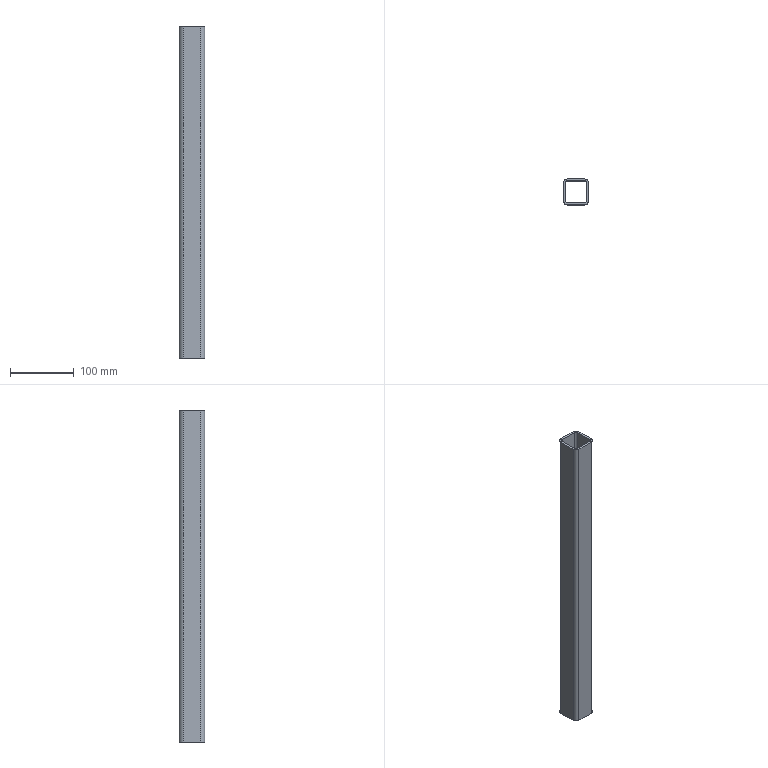Part | STEP file | 3 | 1 solid | 18 faces | box 40 x 40 x 520 mm | volume 217221 mm3 | plane 10 | cylinder 8 | commonest cylinder face diameters 7.2 x4 13.2 x4
STEP:
#1=CARTESIAN_POINT('',(0.,0.,0.));
#2=DIRECTION('',(0.,0.,1.));
#3=DIRECTION('',(1.,0.,0.));
#4=AXIS2_PLACEMENT_3D('',#1,#2,#3);
#5=CARTESIAN_POINT('',(-13.4,-17.,520.));
#6=VERTEX_POINT('',#5);
#7=CARTESIAN_POINT('',(13.4,-17.,520.));
#8=VERTEX_POINT('',#7);
#9=CARTESIAN_POINT('',(6.7,-17.,520.));
#10=DIRECTION('',(1.,0.,0.));
#11=VECTOR('',#10,1.);
#12=LINE('',#9,#11);
#13=CARTESIAN_POINT('',(13.4,-17.,0.));
#14=DIRECTION('',(0.,-1.,0.));
#15=DIRECTION('',(0.,0.,-1.));
#16=AXIS2_PLACEMENT_3D('',#13,#14,#15);
#17=PLANE('',#16);
#18=CARTESIAN_POINT('',(-520.,-6.7));
#19=DIRECTION('',(0.,1.));
#20=VECTOR('',#19,1.);
#21=LINE('',#18,#20);
#22=(GEOMETRIC_REPRESENTATION_CONTEXT(2)PARAMETRIC_REPRESENTATION_CONTEXT()REPRESENTATION_CONTEXT('',''));
#23=DEFINITIONAL_REPRESENTATION('',(#21),#22);
#24=PCURVE('',#17,#23);
#25=CARTESIAN_POINT('',(0.,0.,520.));
#26=DIRECTION('',(0.,0.,1.));
#27=DIRECTION('',(1.,0.,0.));
#28=AXIS2_PLACEMENT_3D('',#25,#26,#27);
#29=PLANE('',#28);
#30=CARTESIAN_POINT('',(6.7,-17.));
#31=DIRECTION('',(1.,0.));
#32=VECTOR('',#31,1.);
#33=LINE('',#30,#32);
#34=(GEOMETRIC_REPRESENTATION_CONTEXT(2)PARAMETRIC_REPRESENTATION_CONTEXT()REPRESENTATION_CONTEXT('',''));
#35=DEFINITIONAL_REPRESENTATION('',(#33),#34);
#36=PCURVE('',#29,#35);
#37=SURFACE_CURVE('',#12,(#24,#36),.PCURVE_S1.);
#38=EDGE_CURVE('',#6,#8,#37,.T.);
#39=ORIENTED_EDGE('',*,*,#38,.T.);
#40=CARTESIAN_POINT('',(13.4,-17.,0.));
#41=VERTEX_POINT('',#40);
#42=CARTESIAN_POINT('',(13.4,-17.,0.));
#43=DIRECTION('',(0.,0.,1.));
#44=VECTOR('',#43,1.);
#45=LINE('',#42,#44);
#46=CARTESIAN_POINT('',(0.,0.));
#47=DIRECTION('',(-1.,0.));
#48=VECTOR('',#47,1.);
#49=LINE('',#46,#48);
#50=(GEOMETRIC_REPRESENTATION_CONTEXT(2)PARAMETRIC_REPRESENTATION_CONTEXT()REPRESENTATION_CONTEXT('',''));
#51=DEFINITIONAL_REPRESENTATION('',(#49),#50);
#52=PCURVE('',#17,#51);
#53=CARTESIAN_POINT('',(13.4,-13.4,0.));
#54=DIRECTION('',(0.,0.,1.));
#55=DIRECTION('',(0.,1.,0.));
#56=AXIS2_PLACEMENT_3D('',#53,#54,#55);
#57=CYLINDRICAL_SURFACE('',#56,3.6);
#58=CARTESIAN_POINT('',(3.142,0.));
#59=DIRECTION('',(0.,1.));
#60=VECTOR('',#59,1.);
#61=LINE('',#58,#60);
#62=(GEOMETRIC_REPRESENTATION_CONTEXT(2)PARAMETRIC_REPRESENTATION_CONTEXT()REPRESENTATION_CONTEXT('',''));
#63=DEFINITIONAL_REPRESENTATION('',(#61),#62);
#64=PCURVE('',#57,#63);
#65=SURFACE_CURVE('',#45,(#52,#64),.PCURVE_S1.);
#66=EDGE_CURVE('',#41,#8,#65,.T.);
#67=ORIENTED_EDGE('',*,*,#66,.F.);
#68=CARTESIAN_POINT('',(-13.4,-17.,0.));
#69=VERTEX_POINT('',#68);
#70=CARTESIAN_POINT('',(6.7,-17.,0.));
#71=DIRECTION('',(1.,0.,0.));
#72=VECTOR('',#71,1.);
#73=LINE('',#70,#72);
#74=CARTESIAN_POINT('',(0.,-6.7));
#75=DIRECTION('',(0.,1.));
#76=VECTOR('',#75,1.);
#77=LINE('',#74,#76);
#78=(GEOMETRIC_REPRESENTATION_CONTEXT(2)PARAMETRIC_REPRESENTATION_CONTEXT()REPRESENTATION_CONTEXT('',''));
#79=DEFINITIONAL_REPRESENTATION('',(#77),#78);
#80=PCURVE('',#17,#79);
#81=CARTESIAN_POINT('',(0.,0.,0.));
#82=DIRECTION('',(0.,0.,1.));
#83=DIRECTION('',(1.,0.,0.));
#84=AXIS2_PLACEMENT_3D('',#81,#82,#83);
#85=PLANE('',#84);
#86=CARTESIAN_POINT('',(6.7,-17.));
#87=DIRECTION('',(1.,0.));
#88=VECTOR('',#87,1.);
#89=LINE('',#86,#88);
#90=(GEOMETRIC_REPRESENTATION_CONTEXT(2)PARAMETRIC_REPRESENTATION_CONTEXT()REPRESENTATION_CONTEXT('',''));
#91=DEFINITIONAL_REPRESENTATION('',(#89),#90);
#92=PCURVE('',#85,#91);
#93=SURFACE_CURVE('',#73,(#80,#92),.PCURVE_S1.);
#94=EDGE_CURVE('',#69,#41,#93,.T.);
#95=ORIENTED_EDGE('',*,*,#94,.F.);
#96=CARTESIAN_POINT('',(-13.4,-17.,0.));
#97=DIRECTION('',(0.,0.,1.));
#98=VECTOR('',#97,1.);
#99=LINE('',#96,#98);
#100=CARTESIAN_POINT('',(0.,-26.8));
#101=DIRECTION('',(-1.,0.));
#102=VECTOR('',#101,1.);
#103=LINE('',#100,#102);
#104=(GEOMETRIC_REPRESENTATION_CONTEXT(2)PARAMETRIC_REPRESENTATION_CONTEXT()REPRESENTATION_CONTEXT('',''));
#105=DEFINITIONAL_REPRESENTATION('',(#103),#104);
#106=PCURVE('',#17,#105);
#107=CARTESIAN_POINT('',(-13.4,-13.4,0.));
#108=DIRECTION('',(0.,0.,1.));
#109=DIRECTION('',(1.,0.,0.));
#110=AXIS2_PLACEMENT_3D('',#107,#108,#109);
#111=CYLINDRICAL_SURFACE('',#110,3.6);
#112=CARTESIAN_POINT('',(4.712,0.));
#113=DIRECTION('',(0.,1.));
#114=VECTOR('',#113,1.);
#115=LINE('',#112,#114);
#116=(GEOMETRIC_REPRESENTATION_CONTEXT(2)PARAMETRIC_REPRESENTATION_CONTEXT()REPRESENTATION_CONTEXT('',''));
#117=DEFINITIONAL_REPRESENTATION('',(#115),#116);
#118=PCURVE('',#111,#117);
#119=SURFACE_CURVE('',#99,(#106,#118),.PCURVE_S1.);
#120=EDGE_CURVE('',#69,#6,#119,.T.);
#121=ORIENTED_EDGE('',*,*,#120,.T.);
#122=EDGE_LOOP('',(#39,#67,#95,#121));
#123=FACE_BOUND('',#122,.T.);
#124=ADVANCED_FACE('',(#123),#17,.F.);
#125=ORIENTED_EDGE('',*,*,#66,.F.);
#126=CARTESIAN_POINT('',(17.,-13.4,0.));
#127=VERTEX_POINT('',#126);
#128=CARTESIAN_POINT('',(13.4,-13.4,0.));
#129=DIRECTION('',(0.,0.,1.));
#130=DIRECTION('',(0.,1.,0.));
#131=AXIS2_PLACEMENT_3D('',#128,#129,#130);
#132=CIRCLE('',#131,3.6);
#133=CARTESIAN_POINT('',(0.,0.));
#134=DIRECTION('',(1.,0.));
#135=VECTOR('',#134,1.);
#136=LINE('',#133,#135);
#137=(GEOMETRIC_REPRESENTATION_CONTEXT(2)PARAMETRIC_REPRESENTATION_CONTEXT()REPRESENTATION_CONTEXT('',''));
#138=DEFINITIONAL_REPRESENTATION('',(#136),#137);
#139=PCURVE('',#57,#138);
#140=CARTESIAN_POINT('',(13.4,-13.4));
#141=DIRECTION('',(0.,1.));
#142=AXIS2_PLACEMENT_2D('',#140,#141);
#143=CIRCLE('',#142,3.6);
#144=(GEOMETRIC_REPRESENTATION_CONTEXT(2)PARAMETRIC_REPRESENTATION_CONTEXT()REPRESENTATION_CONTEXT('',''));
#145=DEFINITIONAL_REPRESENTATION('',(#143),#144);
#146=PCURVE('',#85,#145);
#147=SURFACE_CURVE('',#132,(#139,#146),.PCURVE_S1.);
#148=EDGE_CURVE('',#41,#127,#147,.T.);
#149=ORIENTED_EDGE('',*,*,#148,.T.);
#150=CARTESIAN_POINT('',(17.,-13.4,520.));
#151=VERTEX_POINT('',#150);
#152=CARTESIAN_POINT('',(17.,-13.4,0.));
#153=DIRECTION('',(0.,0.,1.));
#154=VECTOR('',#153,1.);
#155=LINE('',#152,#154);
#156=CARTESIAN_POINT('',(4.712,0.));
#157=DIRECTION('',(0.,1.));
#158=VECTOR('',#157,1.);
#159=LINE('',#156,#158);
#160=(GEOMETRIC_REPRESENTATION_CONTEXT(2)PARAMETRIC_REPRESENTATION_CONTEXT()REPRESENTATION_CONTEXT('',''));
#161=DEFINITIONAL_REPRESENTATION('',(#159),#160);
#162=PCURVE('',#57,#161);
#163=CARTESIAN_POINT('',(17.,13.4,0.));
#164=DIRECTION('',(1.,0.,0.));
#165=DIRECTION('',(0.,0.,-1.));
#166=AXIS2_PLACEMENT_3D('',#163,#164,#165);
#167=PLANE('',#166);
#168=CARTESIAN_POINT('',(0.,-26.8));
#169=DIRECTION('',(-1.,0.));
#170=VECTOR('',#169,1.);
#171=LINE('',#168,#170);
#172=(GEOMETRIC_REPRESENTATION_CONTEXT(2)PARAMETRIC_REPRESENTATION_CONTEXT()REPRESENTATION_CONTEXT('',''));
#173=DEFINITIONAL_REPRESENTATION('',(#171),#172);
#174=PCURVE('',#167,#173);
#175=SURFACE_CURVE('',#155,(#162,#174),.PCURVE_S1.);
#176=EDGE_CURVE('',#127,#151,#175,.T.);
#177=ORIENTED_EDGE('',*,*,#176,.T.);
#178=CARTESIAN_POINT('',(13.4,-13.4,520.));
#179=DIRECTION('',(0.,0.,1.));
#180=DIRECTION('',(0.,1.,0.));
#181=AXIS2_PLACEMENT_3D('',#178,#179,#180);
#182=CIRCLE('',#181,3.6);
#183=CARTESIAN_POINT('',(0.,520.));
#184=DIRECTION('',(1.,0.));
#185=VECTOR('',#184,1.);
#186=LINE('',#183,#185);
#187=(GEOMETRIC_REPRESENTATION_CONTEXT(2)PARAMETRIC_REPRESENTATION_CONTEXT()REPRESENTATION_CONTEXT('',''));
#188=DEFINITIONAL_REPRESENTATION('',(#186),#187);
#189=PCURVE('',#57,#188);
#190=CARTESIAN_POINT('',(13.4,-13.4));
#191=DIRECTION('',(0.,1.));
#192=AXIS2_PLACEMENT_2D('',#190,#191);
#193=CIRCLE('',#192,3.6);
#194=(GEOMETRIC_REPRESENTATION_CONTEXT(2)PARAMETRIC_REPRESENTATION_CONTEXT()REPRESENTATION_CONTEXT('',''));
#195=DEFINITIONAL_REPRESENTATION('',(#193),#194);
#196=PCURVE('',#29,#195);
#197=SURFACE_CURVE('',#182,(#189,#196),.PCURVE_S1.);
#198=EDGE_CURVE('',#8,#151,#197,.T.);
#199=ORIENTED_EDGE('',*,*,#198,.F.);
#200=EDGE_LOOP('',(#125,#149,#177,#199));
#201=FACE_BOUND('',#200,.F.);
#202=ADVANCED_FACE('',(#201),#57,.F.);
#203=CARTESIAN_POINT('',(17.,13.4,520.));
#204=VERTEX_POINT('',#203);
#205=CARTESIAN_POINT('',(17.,6.7,520.));
#206=DIRECTION('',(0.,1.,0.));
#207=VECTOR('',#206,1.);
#208=LINE('',#205,#207);
#209=CARTESIAN_POINT('',(-520.,-6.7));
#210=DIRECTION('',(0.,1.));
#211=VECTOR('',#210,1.);
#212=LINE('',#209,#211);
#213=(GEOMETRIC_REPRESENTATION_CONTEXT(2)PARAMETRIC_REPRESENTATION_CONTEXT()REPRESENTATION_CONTEXT('',''));
#214=DEFINITIONAL_REPRESENTATION('',(#212),#213);
#215=PCURVE('',#167,#214);
#216=CARTESIAN_POINT('',(17.,6.7));
#217=DIRECTION('',(0.,1.));
#218=VECTOR('',#217,1.);
#219=LINE('',#216,#218);
#220=(GEOMETRIC_REPRESENTATION_CONTEXT(2)PARAMETRIC_REPRESENTATION_CONTEXT()REPRESENTATION_CONTEXT('',''));
#221=DEFINITIONAL_REPRESENTATION('',(#219),#220);
#222=PCURVE('',#29,#221);
#223=SURFACE_CURVE('',#208,(#215,#222),.PCURVE_S1.);
#224=EDGE_CURVE('',#151,#204,#223,.T.);
#225=ORIENTED_EDGE('',*,*,#224,.T.);
#226=CARTESIAN_POINT('',(17.,13.4,0.));
#227=VERTEX_POINT('',#226);
#228=CARTESIAN_POINT('',(17.,13.4,0.));
#229=DIRECTION('',(0.,0.,1.));
#230=VECTOR('',#229,1.);
#231=LINE('',#228,#230);
#232=CARTESIAN_POINT('',(0.,0.));
#233=DIRECTION('',(-1.,0.));
#234=VECTOR('',#233,1.);
#235=LINE('',#232,#234);
#236=(GEOMETRIC_REPRESENTATION_CONTEXT(2)PARAMETRIC_REPRESENTATION_CONTEXT()REPRESENTATION_CONTEXT('',''));
#237=DEFINITIONAL_REPRESENTATION('',(#235),#236);
#238=PCURVE('',#167,#237);
#239=CARTESIAN_POINT('',(13.4,13.4,0.));
#240=DIRECTION('',(0.,0.,1.));
#241=DIRECTION('',(-1.,0.,0.));
#242=AXIS2_PLACEMENT_3D('',#239,#240,#241);
#243=CYLINDRICAL_SURFACE('',#242,3.6);
#244=CARTESIAN_POINT('',(3.142,0.));
#245=DIRECTION('',(0.,1.));
#246=VECTOR('',#245,1.);
#247=LINE('',#244,#246);
#248=(GEOMETRIC_REPRESENTATION_CONTEXT(2)PARAMETRIC_REPRESENTATION_CONTEXT()REPRESENTATION_CONTEXT('',''));
#249=DEFINITIONAL_REPRESENTATION('',(#247),#248);
#250=PCURVE('',#243,#249);
#251=SURFACE_CURVE('',#231,(#238,#250),.PCURVE_S1.);
#252=EDGE_CURVE('',#227,#204,#251,.T.);
#253=ORIENTED_EDGE('',*,*,#252,.F.);
#254=CARTESIAN_POINT('',(17.,6.7,0.));
#255=DIRECTION('',(0.,1.,0.));
#256=VECTOR('',#255,1.);
#257=LINE('',#254,#256);
#258=CARTESIAN_POINT('',(0.,-6.7));
#259=DIRECTION('',(0.,1.));
#260=VECTOR('',#259,1.);
#261=LINE('',#258,#260);
#262=(GEOMETRIC_REPRESENTATION_CONTEXT(2)PARAMETRIC_REPRESENTATION_CONTEXT()REPRESENTATION_CONTEXT('',''));
#263=DEFINITIONAL_REPRESENTATION('',(#261),#262);
#264=PCURVE('',#167,#263);
#265=CARTESIAN_POINT('',(17.,6.7));
#266=DIRECTION('',(0.,1.));
#267=VECTOR('',#266,1.);
#268=LINE('',#265,#267);
#269=(GEOMETRIC_REPRESENTATION_CONTEXT(2)PARAMETRIC_REPRESENTATION_CONTEXT()REPRESENTATION_CONTEXT('',''));
#270=DEFINITIONAL_REPRESENTATION('',(#268),#269);
#271=PCURVE('',#85,#270);
#272=SURFACE_CURVE('',#257,(#264,#271),.PCURVE_S1.);
#273=EDGE_CURVE('',#127,#227,#272,.T.);
#274=ORIENTED_EDGE('',*,*,#273,.F.);
#275=ORIENTED_EDGE('',*,*,#176,.T.);
#276=EDGE_LOOP('',(#225,#253,#274,#275));
#277=FACE_BOUND('',#276,.T.);
#278=ADVANCED_FACE('',(#277),#167,.F.);
#279=ORIENTED_EDGE('',*,*,#252,.F.);
#280=CARTESIAN_POINT('',(13.4,17.,0.));
#281=VERTEX_POINT('',#280);
#282=CARTESIAN_POINT('',(13.4,13.4,0.));
#283=DIRECTION('',(0.,0.,1.));
#284=DIRECTION('',(-1.,0.,0.));
#285=AXIS2_PLACEMENT_3D('',#282,#283,#284);
#286=CIRCLE('',#285,3.6);
#287=CARTESIAN_POINT('',(0.,0.));
#288=DIRECTION('',(1.,0.));
#289=VECTOR('',#288,1.);
#290=LINE('',#287,#289);
#291=(GEOMETRIC_REPRESENTATION_CONTEXT(2)PARAMETRIC_REPRESENTATION_CONTEXT()REPRESENTATION_CONTEXT('',''));
#292=DEFINITIONAL_REPRESENTATION('',(#290),#291);
#293=PCURVE('',#243,#292);
#294=CARTESIAN_POINT('',(13.4,13.4));
#295=DIRECTION('',(-1.,0.));
#296=AXIS2_PLACEMENT_2D('',#294,#295);
#297=CIRCLE('',#296,3.6);
#298=(GEOMETRIC_REPRESENTATION_CONTEXT(2)PARAMETRIC_REPRESENTATION_CONTEXT()REPRESENTATION_CONTEXT('',''));
#299=DEFINITIONAL_REPRESENTATION('',(#297),#298);
#300=PCURVE('',#85,#299);
#301=SURFACE_CURVE('',#286,(#293,#300),.PCURVE_S1.);
#302=EDGE_CURVE('',#227,#281,#301,.T.);
#303=ORIENTED_EDGE('',*,*,#302,.T.);
#304=CARTESIAN_POINT('',(13.4,17.,520.));
#305=VERTEX_POINT('',#304);
#306=CARTESIAN_POINT('',(13.4,17.,0.));
#307=DIRECTION('',(0.,0.,1.));
#308=VECTOR('',#307,1.);
#309=LINE('',#306,#308);
#310=CARTESIAN_POINT('',(4.712,0.));
#311=DIRECTION('',(0.,1.));
#312=VECTOR('',#311,1.);
#313=LINE('',#310,#312);
#314=(GEOMETRIC_REPRESENTATION_CONTEXT(2)PARAMETRIC_REPRESENTATION_CONTEXT()REPRESENTATION_CONTEXT('',''));
#315=DEFINITIONAL_REPRESENTATION('',(#313),#314);
#316=PCURVE('',#243,#315);
#317=CARTESIAN_POINT('',(-13.4,17.,0.));
#318=DIRECTION('',(0.,1.,0.));
#319=DIRECTION('',(0.,0.,1.));
#320=AXIS2_PLACEMENT_3D('',#317,#318,#319);
#321=PLANE('',#320);
#322=CARTESIAN_POINT('',(0.,26.8));
#323=DIRECTION('',(1.,0.));
#324=VECTOR('',#323,1.);
#325=LINE('',#322,#324);
#326=(GEOMETRIC_REPRESENTATION_CONTEXT(2)PARAMETRIC_REPRESENTATION_CONTEXT()REPRESENTATION_CONTEXT('',''));
#327=DEFINITIONAL_REPRESENTATION('',(#325),#326);
#328=PCURVE('',#321,#327);
#329=SURFACE_CURVE('',#309,(#316,#328),.PCURVE_S1.);
#330=EDGE_CURVE('',#281,#305,#329,.T.);
#331=ORIENTED_EDGE('',*,*,#330,.T.);
#332=CARTESIAN_POINT('',(13.4,13.4,520.));
#333=DIRECTION('',(0.,0.,1.));
#334=DIRECTION('',(-1.,0.,0.));
#335=AXIS2_PLACEMENT_3D('',#332,#333,#334);
#336=CIRCLE('',#335,3.6);
#337=CARTESIAN_POINT('',(0.,520.));
#338=DIRECTION('',(1.,0.));
#339=VECTOR('',#338,1.);
#340=LINE('',#337,#339);
#341=(GEOMETRIC_REPRESENTATION_CONTEXT(2)PARAMETRIC_REPRESENTATION_CONTEXT()REPRESENTATION_CONTEXT('',''));
#342=DEFINITIONAL_REPRESENTATION('',(#340),#341);
#343=PCURVE('',#243,#342);
#344=CARTESIAN_POINT('',(13.4,13.4));
#345=DIRECTION('',(-1.,0.));
#346=AXIS2_PLACEMENT_2D('',#344,#345);
#347=CIRCLE('',#346,3.6);
#348=(GEOMETRIC_REPRESENTATION_CONTEXT(2)PARAMETRIC_REPRESENTATION_CONTEXT()REPRESENTATION_CONTEXT('',''));
#349=DEFINITIONAL_REPRESENTATION('',(#347),#348);
#350=PCURVE('',#29,#349);
#351=SURFACE_CURVE('',#336,(#343,#350),.PCURVE_S1.);
#352=EDGE_CURVE('',#204,#305,#351,.T.);
#353=ORIENTED_EDGE('',*,*,#352,.F.);
#354=EDGE_LOOP('',(#279,#303,#331,#353));
#355=FACE_BOUND('',#354,.F.);
#356=ADVANCED_FACE('',(#355),#243,.F.);
#357=CARTESIAN_POINT('',(20.,13.4,520.));
#358=VERTEX_POINT('',#357);
#359=CARTESIAN_POINT('',(20.,-13.4,520.));
#360=VERTEX_POINT('',#359);
#361=CARTESIAN_POINT('',(20.,6.7,520.));
#362=DIRECTION('',(0.,-1.,0.));
#363=VECTOR('',#362,1.);
#364=LINE('',#361,#363);
#365=CARTESIAN_POINT('',(20.,13.4,0.));
#366=DIRECTION('',(1.,0.,0.));
#367=DIRECTION('',(0.,0.,-1.));
#368=AXIS2_PLACEMENT_3D('',#365,#366,#367);
#369=PLANE('',#368);
#370=CARTESIAN_POINT('',(-520.,-6.7));
#371=DIRECTION('',(0.,-1.));
#372=VECTOR('',#371,1.);
#373=LINE('',#370,#372);
#374=(GEOMETRIC_REPRESENTATION_CONTEXT(2)PARAMETRIC_REPRESENTATION_CONTEXT()REPRESENTATION_CONTEXT('',''));
#375=DEFINITIONAL_REPRESENTATION('',(#373),#374);
#376=PCURVE('',#369,#375);
#377=CARTESIAN_POINT('',(20.,6.7));
#378=DIRECTION('',(0.,-1.));
#379=VECTOR('',#378,1.);
#380=LINE('',#377,#379);
#381=(GEOMETRIC_REPRESENTATION_CONTEXT(2)PARAMETRIC_REPRESENTATION_CONTEXT()REPRESENTATION_CONTEXT('',''));
#382=DEFINITIONAL_REPRESENTATION('',(#380),#381);
#383=PCURVE('',#29,#382);
#384=SURFACE_CURVE('',#364,(#376,#383),.PCURVE_S1.);
#385=EDGE_CURVE('',#358,#360,#384,.T.);
#386=ORIENTED_EDGE('',*,*,#385,.T.);
#387=CARTESIAN_POINT('',(20.,-13.4,0.));
#388=VERTEX_POINT('',#387);
#389=CARTESIAN_POINT('',(20.,-13.4,0.));
#390=DIRECTION('',(0.,0.,1.));
#391=VECTOR('',#390,1.);
#392=LINE('',#389,#391);
#393=CARTESIAN_POINT('',(0.,-26.8));
#394=DIRECTION('',(-1.,0.));
#395=VECTOR('',#394,1.);
#396=LINE('',#393,#395);
#397=(GEOMETRIC_REPRESENTATION_CONTEXT(2)PARAMETRIC_REPRESENTATION_CONTEXT()REPRESENTATION_CONTEXT('',''));
#398=DEFINITIONAL_REPRESENTATION('',(#396),#397);
#399=PCURVE('',#369,#398);
#400=CARTESIAN_POINT('',(13.4,-13.4,0.));
#401=DIRECTION('',(0.,0.,1.));
#402=DIRECTION('',(0.,1.,0.));
#403=AXIS2_PLACEMENT_3D('',#400,#401,#402);
#404=CYLINDRICAL_SURFACE('',#403,6.6);
#405=CARTESIAN_POINT('',(4.712,0.));
#406=DIRECTION('',(0.,1.));
#407=VECTOR('',#406,1.);
#408=LINE('',#405,#407);
#409=(GEOMETRIC_REPRESENTATION_CONTEXT(2)PARAMETRIC_REPRESENTATION_CONTEXT()REPRESENTATION_CONTEXT('',''));
#410=DEFINITIONAL_REPRESENTATION('',(#408),#409);
#411=PCURVE('',#404,#410);
#412=SURFACE_CURVE('',#392,(#399,#411),.PCURVE_S1.);
#413=EDGE_CURVE('',#388,#360,#412,.T.);
#414=ORIENTED_EDGE('',*,*,#413,.F.);
#415=CARTESIAN_POINT('',(20.,13.4,0.));
#416=VERTEX_POINT('',#415);
#417=CARTESIAN_POINT('',(20.,6.7,0.));
#418=DIRECTION('',(0.,-1.,0.));
#419=VECTOR('',#418,1.);
#420=LINE('',#417,#419);
#421=CARTESIAN_POINT('',(0.,-6.7));
#422=DIRECTION('',(0.,-1.));
#423=VECTOR('',#422,1.);
#424=LINE('',#421,#423);
#425=(GEOMETRIC_REPRESENTATION_CONTEXT(2)PARAMETRIC_REPRESENTATION_CONTEXT()REPRESENTATION_CONTEXT('',''));
#426=DEFINITIONAL_REPRESENTATION('',(#424),#425);
#427=PCURVE('',#369,#426);
#428=CARTESIAN_POINT('',(20.,6.7));
#429=DIRECTION('',(0.,-1.));
#430=VECTOR('',#429,1.);
#431=LINE('',#428,#430);
#432=(GEOMETRIC_REPRESENTATION_CONTEXT(2)PARAMETRIC_REPRESENTATION_CONTEXT()REPRESENTATION_CONTEXT('',''));
#433=DEFINITIONAL_REPRESENTATION('',(#431),#432);
#434=PCURVE('',#85,#433);
#435=SURFACE_CURVE('',#420,(#427,#434),.PCURVE_S1.);
#436=EDGE_CURVE('',#416,#388,#435,.T.);
#437=ORIENTED_EDGE('',*,*,#436,.F.);
#438=CARTESIAN_POINT('',(20.,13.4,0.));
#439=DIRECTION('',(0.,0.,1.));
#440=VECTOR('',#439,1.);
#441=LINE('',#438,#440);
#442=CARTESIAN_POINT('',(0.,0.));
#443=DIRECTION('',(-1.,0.));
#444=VECTOR('',#443,1.);
#445=LINE('',#442,#444);
#446=(GEOMETRIC_REPRESENTATION_CONTEXT(2)PARAMETRIC_REPRESENTATION_CONTEXT()REPRESENTATION_CONTEXT('',''));
#447=DEFINITIONAL_REPRESENTATION('',(#445),#446);
#448=PCURVE('',#369,#447);
#449=CARTESIAN_POINT('',(13.4,13.4,0.));
#450=DIRECTION('',(0.,0.,1.));
#451=DIRECTION('',(-1.,0.,0.));
#452=AXIS2_PLACEMENT_3D('',#449,#450,#451);
#453=CYLINDRICAL_SURFACE('',#452,6.6);
#454=CARTESIAN_POINT('',(3.142,0.));
#455=DIRECTION('',(0.,1.));
#456=VECTOR('',#455,1.);
#457=LINE('',#454,#456);
#458=(GEOMETRIC_REPRESENTATION_CONTEXT(2)PARAMETRIC_REPRESENTATION_CONTEXT()REPRESENTATION_CONTEXT('',''));
#459=DEFINITIONAL_REPRESENTATION('',(#457),#458);
#460=PCURVE('',#453,#459);
#461=SURFACE_CURVE('',#441,(#448,#460),.PCURVE_S1.);
#462=EDGE_CURVE('',#416,#358,#461,.T.);
#463=ORIENTED_EDGE('',*,*,#462,.T.);
#464=EDGE_LOOP('',(#386,#414,#437,#463));
#465=FACE_BOUND('',#464,.T.);
#466=ADVANCED_FACE('',(#465),#369,.T.);
#467=CARTESIAN_POINT('',(13.4,-20.,520.));
#468=VERTEX_POINT('',#467);
#469=CARTESIAN_POINT('',(13.4,-13.4,520.));
#470=DIRECTION('',(0.,0.,-1.));
#471=DIRECTION('',(0.,1.,0.));
#472=AXIS2_PLACEMENT_3D('',#469,#470,#471);
#473=CIRCLE('',#472,6.6);
#474=CARTESIAN_POINT('',(6.283,520.));
#475=DIRECTION('',(-1.,0.));
#476=VECTOR('',#475,1.);
#477=LINE('',#474,#476);
#478=(GEOMETRIC_REPRESENTATION_CONTEXT(2)PARAMETRIC_REPRESENTATION_CONTEXT()REPRESENTATION_CONTEXT('',''));
#479=DEFINITIONAL_REPRESENTATION('',(#477),#478);
#480=PCURVE('',#404,#479);
#481=CARTESIAN_POINT('',(13.4,-6.8));
#482=CARTESIAN_POINT('',(24.832,-6.8));
#483=CARTESIAN_POINT('',(19.116,-16.7));
#484=CARTESIAN_POINT('',(13.4,-26.6));
#485=CARTESIAN_POINT('',(7.684,-16.7));
#486=CARTESIAN_POINT('',(1.968,-6.8));
#487=CARTESIAN_POINT('',(13.4,-6.8));
#488=(BOUNDED_CURVE()B_SPLINE_CURVE(2,(#481,#482,#483,#484,#485,#486,#487),.UNSPECIFIED.,.T.,.F.)B_SPLINE_CURVE_WITH_KNOTS((1,2,2,2,2,1),(-2.094,0.,2.094,4.189,6.283,8.378),.UNSPECIFIED.)CURVE()GEOMETRIC_REPRESENTATION_ITEM()RATIONAL_B_SPLINE_CURVE((1.,0.5,1.,0.5,1.,0.5,1.))REPRESENTATION_ITEM(''));
#489=(GEOMETRIC_REPRESENTATION_CONTEXT(2)PARAMETRIC_REPRESENTATION_CONTEXT()REPRESENTATION_CONTEXT('',''));
#490=DEFINITIONAL_REPRESENTATION('',(#488),#489);
#491=PCURVE('',#29,#490);
#492=SURFACE_CURVE('',#473,(#480,#491),.PCURVE_S1.);
#493=EDGE_CURVE('',#360,#468,#492,.T.);
#494=ORIENTED_EDGE('',*,*,#493,.T.);
#495=CARTESIAN_POINT('',(13.4,-20.,0.));
#496=VERTEX_POINT('',#495);
#497=CARTESIAN_POINT('',(13.4,-20.,0.));
#498=DIRECTION('',(0.,0.,1.));
#499=VECTOR('',#498,1.);
#500=LINE('',#497,#499);
#501=CARTESIAN_POINT('',(3.142,0.));
#502=DIRECTION('',(0.,1.));
#503=VECTOR('',#502,1.);
#504=LINE('',#501,#503);
#505=(GEOMETRIC_REPRESENTATION_CONTEXT(2)PARAMETRIC_REPRESENTATION_CONTEXT()REPRESENTATION_CONTEXT('',''));
#506=DEFINITIONAL_REPRESENTATION('',(#504),#505);
#507=PCURVE('',#404,#506);
#508=CARTESIAN_POINT('',(13.4,-20.,0.));
#509=DIRECTION('',(0.,-1.,0.));
#510=DIRECTION('',(0.,0.,-1.));
#511=AXIS2_PLACEMENT_3D('',#508,#509,#510);
#512=PLANE('',#511);
#513=CARTESIAN_POINT('',(0.,0.));
#514=DIRECTION('',(-1.,0.));
#515=VECTOR('',#514,1.);
#516=LINE('',#513,#515);
#517=(GEOMETRIC_REPRESENTATION_CONTEXT(2)PARAMETRIC_REPRESENTATION_CONTEXT()REPRESENTATION_CONTEXT('',''));
#518=DEFINITIONAL_REPRESENTATION('',(#516),#517);
#519=PCURVE('',#512,#518);
#520=SURFACE_CURVE('',#500,(#507,#519),.PCURVE_S1.);
#521=EDGE_CURVE('',#496,#468,#520,.T.);
#522=ORIENTED_EDGE('',*,*,#521,.F.);
#523=CARTESIAN_POINT('',(13.4,-13.4,0.));
#524=DIRECTION('',(0.,0.,-1.));
#525=DIRECTION('',(0.,1.,0.));
#526=AXIS2_PLACEMENT_3D('',#523,#524,#525);
#527=CIRCLE('',#526,6.6);
#528=CARTESIAN_POINT('',(6.283,0.));
#529=DIRECTION('',(-1.,0.));
#530=VECTOR('',#529,1.);
#531=LINE('',#528,#530);
#532=(GEOMETRIC_REPRESENTATION_CONTEXT(2)PARAMETRIC_REPRESENTATION_CONTEXT()REPRESENTATION_CONTEXT('',''));
#533=DEFINITIONAL_REPRESENTATION('',(#531),#532);
#534=PCURVE('',#404,#533);
#535=CARTESIAN_POINT('',(13.4,-6.8));
#536=CARTESIAN_POINT('',(24.832,-6.8));
#537=CARTESIAN_POINT('',(19.116,-16.7));
#538=CARTESIAN_POINT('',(13.4,-26.6));
#539=CARTESIAN_POINT('',(7.684,-16.7));
#540=CARTESIAN_POINT('',(1.968,-6.8));
#541=CARTESIAN_POINT('',(13.4,-6.8));
#542=(BOUNDED_CURVE()B_SPLINE_CURVE(2,(#535,#536,#537,#538,#539,#540,#541),.UNSPECIFIED.,.T.,.F.)B_SPLINE_CURVE_WITH_KNOTS((1,2,2,2,2,1),(-2.094,0.,2.094,4.189,6.283,8.378),.UNSPECIFIED.)CURVE()GEOMETRIC_REPRESENTATION_ITEM()RATIONAL_B_SPLINE_CURVE((1.,0.5,1.,0.5,1.,0.5,1.))REPRESENTATION_ITEM(''));
#543=(GEOMETRIC_REPRESENTATION_CONTEXT(2)PARAMETRIC_REPRESENTATION_CONTEXT()REPRESENTATION_CONTEXT('',''));
#544=DEFINITIONAL_REPRESENTATION('',(#542),#543);
#545=PCURVE('',#85,#544);
#546=SURFACE_CURVE('',#527,(#534,#545),.PCURVE_S1.);
#547=EDGE_CURVE('',#388,#496,#546,.T.);
#548=ORIENTED_EDGE('',*,*,#547,.F.);
#549=ORIENTED_EDGE('',*,*,#413,.T.);
#550=EDGE_LOOP('',(#494,#522,#548,#549));
#551=FACE_BOUND('',#550,.T.);
#552=ADVANCED_FACE('',(#551),#404,.T.);
#553=CARTESIAN_POINT('',(-13.4,-20.,520.));
#554=VERTEX_POINT('',#553);
#555=CARTESIAN_POINT('',(6.7,-20.,520.));
#556=DIRECTION('',(-1.,0.,0.));
#557=VECTOR('',#556,1.);
#558=LINE('',#555,#557);
#559=CARTESIAN_POINT('',(-520.,-6.7));
#560=DIRECTION('',(0.,-1.));
#561=VECTOR('',#560,1.);
#562=LINE('',#559,#561);
#563=(GEOMETRIC_REPRESENTATION_CONTEXT(2)PARAMETRIC_REPRESENTATION_CONTEXT()REPRESENTATION_CONTEXT('',''));
#564=DEFINITIONAL_REPRESENTATION('',(#562),#563);
#565=PCURVE('',#512,#564);
#566=CARTESIAN_POINT('',(6.7,-20.));
#567=DIRECTION('',(-1.,0.));
#568=VECTOR('',#567,1.);
#569=LINE('',#566,#568);
#570=(GEOMETRIC_REPRESENTATION_CONTEXT(2)PARAMETRIC_REPRESENTATION_CONTEXT()REPRESENTATION_CONTEXT('',''));
#571=DEFINITIONAL_REPRESENTATION('',(#569),#570);
#572=PCURVE('',#29,#571);
#573=SURFACE_CURVE('',#558,(#565,#572),.PCURVE_S1.);
#574=EDGE_CURVE('',#468,#554,#573,.T.);
#575=ORIENTED_EDGE('',*,*,#574,.T.);
#576=CARTESIAN_POINT('',(-13.4,-20.,0.));
#577=VERTEX_POINT('',#576);
#578=CARTESIAN_POINT('',(-13.4,-20.,0.));
#579=DIRECTION('',(0.,0.,1.));
#580=VECTOR('',#579,1.);
#581=LINE('',#578,#580);
#582=CARTESIAN_POINT('',(0.,-26.8));
#583=DIRECTION('',(-1.,0.));
#584=VECTOR('',#583,1.);
#585=LINE('',#582,#584);
#586=(GEOMETRIC_REPRESENTATION_CONTEXT(2)PARAMETRIC_REPRESENTATION_CONTEXT()REPRESENTATION_CONTEXT('',''));
#587=DEFINITIONAL_REPRESENTATION('',(#585),#586);
#588=PCURVE('',#512,#587);
#589=CARTESIAN_POINT('',(-13.4,-13.4,0.));
#590=DIRECTION('',(0.,0.,1.));
#591=DIRECTION('',(1.,0.,0.));
#592=AXIS2_PLACEMENT_3D('',#589,#590,#591);
#593=CYLINDRICAL_SURFACE('',#592,6.6);
#594=CARTESIAN_POINT('',(4.712,0.));
#595=DIRECTION('',(0.,1.));
#596=VECTOR('',#595,1.);
#597=LINE('',#594,#596);
#598=(GEOMETRIC_REPRESENTATION_CONTEXT(2)PARAMETRIC_REPRESENTATION_CONTEXT()REPRESENTATION_CONTEXT('',''));
#599=DEFINITIONAL_REPRESENTATION('',(#597),#598);
#600=PCURVE('',#593,#599);
#601=SURFACE_CURVE('',#581,(#588,#600),.PCURVE_S1.);
#602=EDGE_CURVE('',#577,#554,#601,.T.);
#603=ORIENTED_EDGE('',*,*,#602,.F.);
#604=CARTESIAN_POINT('',(6.7,-20.,0.));
#605=DIRECTION('',(-1.,0.,0.));
#606=VECTOR('',#605,1.);
#607=LINE('',#604,#606);
#608=CARTESIAN_POINT('',(0.,-6.7));
#609=DIRECTION('',(0.,-1.));
#610=VECTOR('',#609,1.);
#611=LINE('',#608,#610);
#612=(GEOMETRIC_REPRESENTATION_CONTEXT(2)PARAMETRIC_REPRESENTATION_CONTEXT()REPRESENTATION_CONTEXT('',''));
#613=DEFINITIONAL_REPRESENTATION('',(#611),#612);
#614=PCURVE('',#512,#613);
#615=CARTESIAN_POINT('',(6.7,-20.));
#616=DIRECTION('',(-1.,0.));
#617=VECTOR('',#616,1.);
#618=LINE('',#615,#617);
#619=(GEOMETRIC_REPRESENTATION_CONTEXT(2)PARAMETRIC_REPRESENTATION_CONTEXT()REPRESENTATION_CONTEXT('',''));
#620=DEFINITIONAL_REPRESENTATION('',(#618),#619);
#621=PCURVE('',#85,#620);
#622=SURFACE_CURVE('',#607,(#614,#621),.PCURVE_S1.);
#623=EDGE_CURVE('',#496,#577,#622,.T.);
#624=ORIENTED_EDGE('',*,*,#623,.F.);
#625=ORIENTED_EDGE('',*,*,#521,.T.);
#626=EDGE_LOOP('',(#575,#603,#624,#625));
#627=FACE_BOUND('',#626,.T.);
#628=ADVANCED_FACE('',(#627),#512,.T.);
#629=CARTESIAN_POINT('',(-20.,-13.4,520.));
#630=VERTEX_POINT('',#629);
#631=CARTESIAN_POINT('',(-13.4,-13.4,520.));
#632=DIRECTION('',(0.,0.,-1.));
#633=DIRECTION('',(1.,0.,0.));
#634=AXIS2_PLACEMENT_3D('',#631,#632,#633);
#635=CIRCLE('',#634,6.6);
#636=CARTESIAN_POINT('',(6.283,520.));
#637=DIRECTION('',(-1.,0.));
#638=VECTOR('',#637,1.);
#639=LINE('',#636,#638);
#640=(GEOMETRIC_REPRESENTATION_CONTEXT(2)PARAMETRIC_REPRESENTATION_CONTEXT()REPRESENTATION_CONTEXT('',''));
#641=DEFINITIONAL_REPRESENTATION('',(#639),#640);
#642=PCURVE('',#593,#641);
#643=CARTESIAN_POINT('',(-6.8,-13.4));
#644=CARTESIAN_POINT('',(-6.8,-24.832));
#645=CARTESIAN_POINT('',(-16.7,-19.116));
#646=CARTESIAN_POINT('',(-26.6,-13.4));
#647=CARTESIAN_POINT('',(-16.7,-7.684));
#648=CARTESIAN_POINT('',(-6.8,-1.968));
#649=CARTESIAN_POINT('',(-6.8,-13.4));
#650=(BOUNDED_CURVE()B_SPLINE_CURVE(2,(#643,#644,#645,#646,#647,#648,#649),.UNSPECIFIED.,.T.,.F.)B_SPLINE_CURVE_WITH_KNOTS((1,2,2,2,2,1),(-2.094,0.,2.094,4.189,6.283,8.378),.UNSPECIFIED.)CURVE()GEOMETRIC_REPRESENTATION_ITEM()RATIONAL_B_SPLINE_CURVE((1.,0.5,1.,0.5,1.,0.5,1.))REPRESENTATION_ITEM(''));
#651=(GEOMETRIC_REPRESENTATION_CONTEXT(2)PARAMETRIC_REPRESENTATION_CONTEXT()REPRESENTATION_CONTEXT('',''));
#652=DEFINITIONAL_REPRESENTATION('',(#650),#651);
#653=PCURVE('',#29,#652);
#654=SURFACE_CURVE('',#635,(#642,#653),.PCURVE_S1.);
#655=EDGE_CURVE('',#554,#630,#654,.T.);
#656=ORIENTED_EDGE('',*,*,#655,.T.);
#657=CARTESIAN_POINT('',(-20.,-13.4,0.));
#658=VERTEX_POINT('',#657);
#659=CARTESIAN_POINT('',(-20.,-13.4,0.));
#660=DIRECTION('',(0.,0.,1.));
#661=VECTOR('',#660,1.);
#662=LINE('',#659,#661);
#663=CARTESIAN_POINT('',(3.142,0.));
#664=DIRECTION('',(0.,1.));
#665=VECTOR('',#664,1.);
#666=LINE('',#663,#665);
#667=(GEOMETRIC_REPRESENTATION_CONTEXT(2)PARAMETRIC_REPRESENTATION_CONTEXT()REPRESENTATION_CONTEXT('',''));
#668=DEFINITIONAL_REPRESENTATION('',(#666),#667);
#669=PCURVE('',#593,#668);
#670=CARTESIAN_POINT('',(-20.,-13.4,0.));
#671=DIRECTION('',(-1.,0.,0.));
#672=DIRECTION('',(0.,0.,1.));
#673=AXIS2_PLACEMENT_3D('',#670,#671,#672);
#674=PLANE('',#673);
#675=CARTESIAN_POINT('',(0.,0.));
#676=DIRECTION('',(1.,0.));
#677=VECTOR('',#676,1.);
#678=LINE('',#675,#677);
#679=(GEOMETRIC_REPRESENTATION_CONTEXT(2)PARAMETRIC_REPRESENTATION_CONTEXT()REPRESENTATION_CONTEXT('',''));
#680=DEFINITIONAL_REPRESENTATION('',(#678),#679);
#681=PCURVE('',#674,#680);
#682=SURFACE_CURVE('',#662,(#669,#681),.PCURVE_S1.);
#683=EDGE_CURVE('',#658,#630,#682,.T.);
#684=ORIENTED_EDGE('',*,*,#683,.F.);
#685=CARTESIAN_POINT('',(-13.4,-13.4,0.));
#686=DIRECTION('',(0.,0.,-1.));
#687=DIRECTION('',(1.,0.,0.));
#688=AXIS2_PLACEMENT_3D('',#685,#686,#687);
#689=CIRCLE('',#688,6.6);
#690=CARTESIAN_POINT('',(6.283,0.));
#691=DIRECTION('',(-1.,0.));
#692=VECTOR('',#691,1.);
#693=LINE('',#690,#692);
#694=(GEOMETRIC_REPRESENTATION_CONTEXT(2)PARAMETRIC_REPRESENTATION_CONTEXT()REPRESENTATION_CONTEXT('',''));
#695=DEFINITIONAL_REPRESENTATION('',(#693),#694);
#696=PCURVE('',#593,#695);
#697=CARTESIAN_POINT('',(-6.8,-13.4));
#698=CARTESIAN_POINT('',(-6.8,-24.832));
#699=CARTESIAN_POINT('',(-16.7,-19.116));
#700=CARTESIAN_POINT('',(-26.6,-13.4));
#701=CARTESIAN_POINT('',(-16.7,-7.684));
#702=CARTESIAN_POINT('',(-6.8,-1.968));
#703=CARTESIAN_POINT('',(-6.8,-13.4));
#704=(BOUNDED_CURVE()B_SPLINE_CURVE(2,(#697,#698,#699,#700,#701,#702,#703),.UNSPECIFIED.,.T.,.F.)B_SPLINE_CURVE_WITH_KNOTS((1,2,2,2,2,1),(-2.094,0.,2.094,4.189,6.283,8.378),.UNSPECIFIED.)CURVE()GEOMETRIC_REPRESENTATION_ITEM()RATIONAL_B_SPLINE_CURVE((1.,0.5,1.,0.5,1.,0.5,1.))REPRESENTATION_ITEM(''));
#705=(GEOMETRIC_REPRESENTATION_CONTEXT(2)PARAMETRIC_REPRESENTATION_CONTEXT()REPRESENTATION_CONTEXT('',''));
#706=DEFINITIONAL_REPRESENTATION('',(#704),#705);
#707=PCURVE('',#85,#706);
#708=SURFACE_CURVE('',#689,(#696,#707),.PCURVE_S1.);
#709=EDGE_CURVE('',#577,#658,#708,.T.);
#710=ORIENTED_EDGE('',*,*,#709,.F.);
#711=ORIENTED_EDGE('',*,*,#602,.T.);
#712=EDGE_LOOP('',(#656,#684,#710,#711));
#713=FACE_BOUND('',#712,.T.);
#714=ADVANCED_FACE('',(#713),#593,.T.);
#715=CARTESIAN_POINT('',(-13.4,17.,520.));
#716=VERTEX_POINT('',#715);
#717=CARTESIAN_POINT('',(-6.7,17.,520.));
#718=DIRECTION('',(-1.,0.,0.));
#719=VECTOR('',#718,1.);
#720=LINE('',#717,#719);
#721=CARTESIAN_POINT('',(520.,6.7));
#722=DIRECTION('',(0.,-1.));
#723=VECTOR('',#722,1.);
#724=LINE('',#721,#723);
#725=(GEOMETRIC_REPRESENTATION_CONTEXT(2)PARAMETRIC_REPRESENTATION_CONTEXT()REPRESENTATION_CONTEXT('',''));
#726=DEFINITIONAL_REPRESENTATION('',(#724),#725);
#727=PCURVE('',#321,#726);
#728=CARTESIAN_POINT('',(-6.7,17.));
#729=DIRECTION('',(-1.,0.));
#730=VECTOR('',#729,1.);
#731=LINE('',#728,#730);
#732=(GEOMETRIC_REPRESENTATION_CONTEXT(2)PARAMETRIC_REPRESENTATION_CONTEXT()REPRESENTATION_CONTEXT('',''));
#733=DEFINITIONAL_REPRESENTATION('',(#731),#732);
#734=PCURVE('',#29,#733);
#735=SURFACE_CURVE('',#720,(#727,#734),.PCURVE_S1.);
#736=EDGE_CURVE('',#305,#716,#735,.T.);
#737=ORIENTED_EDGE('',*,*,#736,.T.);
#738=CARTESIAN_POINT('',(-13.4,17.,0.));
#739=VERTEX_POINT('',#738);
#740=CARTESIAN_POINT('',(-13.4,17.,0.));
#741=DIRECTION('',(0.,0.,1.));
#742=VECTOR('',#741,1.);
#743=LINE('',#740,#742);
#744=CARTESIAN_POINT('',(0.,0.));
#745=DIRECTION('',(1.,0.));
#746=VECTOR('',#745,1.);
#747=LINE('',#744,#746);
#748=(GEOMETRIC_REPRESENTATION_CONTEXT(2)PARAMETRIC_REPRESENTATION_CONTEXT()REPRESENTATION_CONTEXT('',''));
#749=DEFINITIONAL_REPRESENTATION('',(#747),#748);
#750=PCURVE('',#321,#749);
#751=CARTESIAN_POINT('',(-13.4,13.4,0.));
#752=DIRECTION('',(0.,0.,1.));
#753=DIRECTION('',(0.,-1.,0.));
#754=AXIS2_PLACEMENT_3D('',#751,#752,#753);
#755=CYLINDRICAL_SURFACE('',#754,3.6);
#756=CARTESIAN_POINT('',(3.142,0.));
#757=DIRECTION('',(0.,1.));
#758=VECTOR('',#757,1.);
#759=LINE('',#756,#758);
#760=(GEOMETRIC_REPRESENTATION_CONTEXT(2)PARAMETRIC_REPRESENTATION_CONTEXT()REPRESENTATION_CONTEXT('',''));
#761=DEFINITIONAL_REPRESENTATION('',(#759),#760);
#762=PCURVE('',#755,#761);
#763=SURFACE_CURVE('',#743,(#750,#762),.PCURVE_S1.);
#764=EDGE_CURVE('',#739,#716,#763,.T.);
#765=ORIENTED_EDGE('',*,*,#764,.F.);
#766=CARTESIAN_POINT('',(-6.7,17.,0.));
#767=DIRECTION('',(-1.,0.,0.));
#768=VECTOR('',#767,1.);
#769=LINE('',#766,#768);
#770=CARTESIAN_POINT('',(0.,6.7));
#771=DIRECTION('',(0.,-1.));
#772=VECTOR('',#771,1.);
#773=LINE('',#770,#772);
#774=(GEOMETRIC_REPRESENTATION_CONTEXT(2)PARAMETRIC_REPRESENTATION_CONTEXT()REPRESENTATION_CONTEXT('',''));
#775=DEFINITIONAL_REPRESENTATION('',(#773),#774);
#776=PCURVE('',#321,#775);
#777=CARTESIAN_POINT('',(-6.7,17.));
#778=DIRECTION('',(-1.,0.));
#779=VECTOR('',#778,1.);
#780=LINE('',#777,#779);
#781=(GEOMETRIC_REPRESENTATION_CONTEXT(2)PARAMETRIC_REPRESENTATION_CONTEXT()REPRESENTATION_CONTEXT('',''));
#782=DEFINITIONAL_REPRESENTATION('',(#780),#781);
#783=PCURVE('',#85,#782);
#784=SURFACE_CURVE('',#769,(#776,#783),.PCURVE_S1.);
#785=EDGE_CURVE('',#281,#739,#784,.T.);
#786=ORIENTED_EDGE('',*,*,#785,.F.);
#787=ORIENTED_EDGE('',*,*,#330,.T.);
#788=EDGE_LOOP('',(#737,#765,#786,#787));
#789=FACE_BOUND('',#788,.T.);
#790=ADVANCED_FACE('',(#789),#321,.F.);
#791=CARTESIAN_POINT('',(-17.,-13.4,0.));
#792=VERTEX_POINT('',#791);
#793=CARTESIAN_POINT('',(-17.,-13.4,520.));
#794=VERTEX_POINT('',#793);
#795=CARTESIAN_POINT('',(-17.,-13.4,0.));
#796=DIRECTION('',(0.,0.,1.));
#797=VECTOR('',#796,1.);
#798=LINE('',#795,#797);
#799=CARTESIAN_POINT('',(3.142,0.));
#800=DIRECTION('',(0.,1.));
#801=VECTOR('',#800,1.);
#802=LINE('',#799,#801);
#803=(GEOMETRIC_REPRESENTATION_CONTEXT(2)PARAMETRIC_REPRESENTATION_CONTEXT()REPRESENTATION_CONTEXT('',''));
#804=DEFINITIONAL_REPRESENTATION('',(#802),#803);
#805=PCURVE('',#111,#804);
#806=CARTESIAN_POINT('',(-17.,-13.4,0.));
#807=DIRECTION('',(-1.,0.,0.));
#808=DIRECTION('',(0.,0.,1.));
#809=AXIS2_PLACEMENT_3D('',#806,#807,#808);
#810=PLANE('',#809);
#811=CARTESIAN_POINT('',(0.,0.));
#812=DIRECTION('',(1.,0.));
#813=VECTOR('',#812,1.);
#814=LINE('',#811,#813);
#815=(GEOMETRIC_REPRESENTATION_CONTEXT(2)PARAMETRIC_REPRESENTATION_CONTEXT()REPRESENTATION_CONTEXT('',''));
#816=DEFINITIONAL_REPRESENTATION('',(#814),#815);
#817=PCURVE('',#810,#816);
#818=SURFACE_CURVE('',#798,(#805,#817),.PCURVE_S1.);
#819=EDGE_CURVE('',#792,#794,#818,.T.);
#820=ORIENTED_EDGE('',*,*,#819,.F.);
#821=CARTESIAN_POINT('',(-13.4,-13.4,0.));
#822=DIRECTION('',(0.,0.,1.));
#823=DIRECTION('',(1.,0.,0.));
#824=AXIS2_PLACEMENT_3D('',#821,#822,#823);
#825=CIRCLE('',#824,3.6);
#826=CARTESIAN_POINT('',(0.,0.));
#827=DIRECTION('',(1.,0.));
#828=VECTOR('',#827,1.);
#829=LINE('',#826,#828);
#830=(GEOMETRIC_REPRESENTATION_CONTEXT(2)PARAMETRIC_REPRESENTATION_CONTEXT()REPRESENTATION_CONTEXT('',''));
#831=DEFINITIONAL_REPRESENTATION('',(#829),#830);
#832=PCURVE('',#111,#831);
#833=CARTESIAN_POINT('',(-13.4,-13.4));
#834=DIRECTION('',(1.,0.));
#835=AXIS2_PLACEMENT_2D('',#833,#834);
#836=CIRCLE('',#835,3.6);
#837=(GEOMETRIC_REPRESENTATION_CONTEXT(2)PARAMETRIC_REPRESENTATION_CONTEXT()REPRESENTATION_CONTEXT('',''));
#838=DEFINITIONAL_REPRESENTATION('',(#836),#837);
#839=PCURVE('',#85,#838);
#840=SURFACE_CURVE('',#825,(#832,#839),.PCURVE_S1.);
#841=EDGE_CURVE('',#792,#69,#840,.T.);
#842=ORIENTED_EDGE('',*,*,#841,.T.);
#843=ORIENTED_EDGE('',*,*,#120,.T.);
#844=CARTESIAN_POINT('',(-13.4,-13.4,520.));
#845=DIRECTION('',(0.,0.,1.));
#846=DIRECTION('',(1.,0.,0.));
#847=AXIS2_PLACEMENT_3D('',#844,#845,#846);
#848=CIRCLE('',#847,3.6);
#849=CARTESIAN_POINT('',(0.,520.));
#850=DIRECTION('',(1.,0.));
#851=VECTOR('',#850,1.);
#852=LINE('',#849,#851);
#853=(GEOMETRIC_REPRESENTATION_CONTEXT(2)PARAMETRIC_REPRESENTATION_CONTEXT()REPRESENTATION_CONTEXT('',''));
#854=DEFINITIONAL_REPRESENTATION('',(#852),#853);
#855=PCURVE('',#111,#854);
#856=CARTESIAN_POINT('',(-13.4,-13.4));
#857=DIRECTION('',(1.,0.));
#858=AXIS2_PLACEMENT_2D('',#856,#857);
#859=CIRCLE('',#858,3.6);
#860=(GEOMETRIC_REPRESENTATION_CONTEXT(2)PARAMETRIC_REPRESENTATION_CONTEXT()REPRESENTATION_CONTEXT('',''));
#861=DEFINITIONAL_REPRESENTATION('',(#859),#860);
#862=PCURVE('',#29,#861);
#863=SURFACE_CURVE('',#848,(#855,#862),.PCURVE_S1.);
#864=EDGE_CURVE('',#794,#6,#863,.T.);
#865=ORIENTED_EDGE('',*,*,#864,.F.);
#866=EDGE_LOOP('',(#820,#842,#843,#865));
#867=FACE_BOUND('',#866,.F.);
#868=ADVANCED_FACE('',(#867),#111,.F.);
#869=CARTESIAN_POINT('',(-17.,13.4,520.));
#870=VERTEX_POINT('',#869);
#871=CARTESIAN_POINT('',(-17.,-6.7,520.));
#872=DIRECTION('',(0.,-1.,0.));
#873=VECTOR('',#872,1.);
#874=LINE('',#871,#873);
#875=CARTESIAN_POINT('',(520.,6.7));
#876=DIRECTION('',(0.,-1.));
#877=VECTOR('',#876,1.);
#878=LINE('',#875,#877);
#879=(GEOMETRIC_REPRESENTATION_CONTEXT(2)PARAMETRIC_REPRESENTATION_CONTEXT()REPRESENTATION_CONTEXT('',''));
#880=DEFINITIONAL_REPRESENTATION('',(#878),#879);
#881=PCURVE('',#810,#880);
#882=CARTESIAN_POINT('',(-17.,-6.7));
#883=DIRECTION('',(0.,-1.));
#884=VECTOR('',#883,1.);
#885=LINE('',#882,#884);
#886=(GEOMETRIC_REPRESENTATION_CONTEXT(2)PARAMETRIC_REPRESENTATION_CONTEXT()REPRESENTATION_CONTEXT('',''));
#887=DEFINITIONAL_REPRESENTATION('',(#885),#886);
#888=PCURVE('',#29,#887);
#889=SURFACE_CURVE('',#874,(#881,#888),.PCURVE_S1.);
#890=EDGE_CURVE('',#870,#794,#889,.T.);
#891=ORIENTED_EDGE('',*,*,#890,.T.);
#892=ORIENTED_EDGE('',*,*,#819,.F.);
#893=CARTESIAN_POINT('',(-17.,13.4,0.));
#894=VERTEX_POINT('',#893);
#895=CARTESIAN_POINT('',(-17.,-6.7,0.));
#896=DIRECTION('',(0.,-1.,0.));
#897=VECTOR('',#896,1.);
#898=LINE('',#895,#897);
#899=CARTESIAN_POINT('',(0.,6.7));
#900=DIRECTION('',(0.,-1.));
#901=VECTOR('',#900,1.);
#902=LINE('',#899,#901);
#903=(GEOMETRIC_REPRESENTATION_CONTEXT(2)PARAMETRIC_REPRESENTATION_CONTEXT()REPRESENTATION_CONTEXT('',''));
#904=DEFINITIONAL_REPRESENTATION('',(#902),#903);
#905=PCURVE('',#810,#904);
#906=CARTESIAN_POINT('',(-17.,-6.7));
#907=DIRECTION('',(0.,-1.));
#908=VECTOR('',#907,1.);
#909=LINE('',#906,#908);
#910=(GEOMETRIC_REPRESENTATION_CONTEXT(2)PARAMETRIC_REPRESENTATION_CONTEXT()REPRESENTATION_CONTEXT('',''));
#911=DEFINITIONAL_REPRESENTATION('',(#909),#910);
#912=PCURVE('',#85,#911);
#913=SURFACE_CURVE('',#898,(#905,#912),.PCURVE_S1.);
#914=EDGE_CURVE('',#894,#792,#913,.T.);
#915=ORIENTED_EDGE('',*,*,#914,.F.);
#916=CARTESIAN_POINT('',(-17.,13.4,0.));
#917=DIRECTION('',(0.,0.,1.));
#918=VECTOR('',#917,1.);
#919=LINE('',#916,#918);
#920=CARTESIAN_POINT('',(0.,26.8));
#921=DIRECTION('',(1.,0.));
#922=VECTOR('',#921,1.);
#923=LINE('',#920,#922);
#924=(GEOMETRIC_REPRESENTATION_CONTEXT(2)PARAMETRIC_REPRESENTATION_CONTEXT()REPRESENTATION_CONTEXT('',''));
#925=DEFINITIONAL_REPRESENTATION('',(#923),#924);
#926=PCURVE('',#810,#925);
#927=CARTESIAN_POINT('',(4.712,0.));
#928=DIRECTION('',(0.,1.));
#929=VECTOR('',#928,1.);
#930=LINE('',#927,#929);
#931=(GEOMETRIC_REPRESENTATION_CONTEXT(2)PARAMETRIC_REPRESENTATION_CONTEXT()REPRESENTATION_CONTEXT('',''));
#932=DEFINITIONAL_REPRESENTATION('',(#930),#931);
#933=PCURVE('',#755,#932);
#934=SURFACE_CURVE('',#919,(#926,#933),.PCURVE_S1.);
#935=EDGE_CURVE('',#894,#870,#934,.T.);
#936=ORIENTED_EDGE('',*,*,#935,.T.);
#937=EDGE_LOOP('',(#891,#892,#915,#936));
#938=FACE_BOUND('',#937,.T.);
#939=ADVANCED_FACE('',(#938),#810,.F.);
#940=ORIENTED_EDGE('',*,*,#764,.F.);
#941=CARTESIAN_POINT('',(-13.4,13.4,0.));
#942=DIRECTION('',(0.,0.,1.));
#943=DIRECTION('',(0.,-1.,0.));
#944=AXIS2_PLACEMENT_3D('',#941,#942,#943);
#945=CIRCLE('',#944,3.6);
#946=CARTESIAN_POINT('',(0.,0.));
#947=DIRECTION('',(1.,0.));
#948=VECTOR('',#947,1.);
#949=LINE('',#946,#948);
#950=(GEOMETRIC_REPRESENTATION_CONTEXT(2)PARAMETRIC_REPRESENTATION_CONTEXT()REPRESENTATION_CONTEXT('',''));
#951=DEFINITIONAL_REPRESENTATION('',(#949),#950);
#952=PCURVE('',#755,#951);
#953=CARTESIAN_POINT('',(-13.4,13.4));
#954=DIRECTION('',(0.,-1.));
#955=AXIS2_PLACEMENT_2D('',#953,#954);
#956=CIRCLE('',#955,3.6);
#957=(GEOMETRIC_REPRESENTATION_CONTEXT(2)PARAMETRIC_REPRESENTATION_CONTEXT()REPRESENTATION_CONTEXT('',''));
#958=DEFINITIONAL_REPRESENTATION('',(#956),#957);
#959=PCURVE('',#85,#958);
#960=SURFACE_CURVE('',#945,(#952,#959),.PCURVE_S1.);
#961=EDGE_CURVE('',#739,#894,#960,.T.);
#962=ORIENTED_EDGE('',*,*,#961,.T.);
#963=ORIENTED_EDGE('',*,*,#935,.T.);
#964=CARTESIAN_POINT('',(-13.4,13.4,520.));
#965=DIRECTION('',(0.,0.,1.));
#966=DIRECTION('',(0.,-1.,0.));
#967=AXIS2_PLACEMENT_3D('',#964,#965,#966);
#968=CIRCLE('',#967,3.6);
#969=CARTESIAN_POINT('',(0.,520.));
#970=DIRECTION('',(1.,0.));
#971=VECTOR('',#970,1.);
#972=LINE('',#969,#971);
#973=(GEOMETRIC_REPRESENTATION_CONTEXT(2)PARAMETRIC_REPRESENTATION_CONTEXT()REPRESENTATION_CONTEXT('',''));
#974=DEFINITIONAL_REPRESENTATION('',(#972),#973);
#975=PCURVE('',#755,#974);
#976=CARTESIAN_POINT('',(-13.4,13.4));
#977=DIRECTION('',(0.,-1.));
#978=AXIS2_PLACEMENT_2D('',#976,#977);
#979=CIRCLE('',#978,3.6);
#980=(GEOMETRIC_REPRESENTATION_CONTEXT(2)PARAMETRIC_REPRESENTATION_CONTEXT()REPRESENTATION_CONTEXT('',''));
#981=DEFINITIONAL_REPRESENTATION('',(#979),#980);
#982=PCURVE('',#29,#981);
#983=SURFACE_CURVE('',#968,(#975,#982),.PCURVE_S1.);
#984=EDGE_CURVE('',#716,#870,#983,.T.);
#985=ORIENTED_EDGE('',*,*,#984,.F.);
#986=EDGE_LOOP('',(#940,#962,#963,#985));
#987=FACE_BOUND('',#986,.F.);
#988=ADVANCED_FACE('',(#987),#755,.F.);
#989=CARTESIAN_POINT('',(-20.,13.4,520.));
#990=VERTEX_POINT('',#989);
#991=CARTESIAN_POINT('',(-20.,-6.7,520.));
#992=DIRECTION('',(0.,1.,0.));
#993=VECTOR('',#992,1.);
#994=LINE('',#991,#993);
#995=CARTESIAN_POINT('',(520.,6.7));
#996=DIRECTION('',(0.,1.));
#997=VECTOR('',#996,1.);
#998=LINE('',#995,#997);
#999=(GEOMETRIC_REPRESENTATION_CONTEXT(2)PARAMETRIC_REPRESENTATION_CONTEXT()REPRESENTATION_CONTEXT('',''));
#1000=DEFINITIONAL_REPRESENTATION('',(#998),#999);
#1001=PCURVE('',#674,#1000);
#1002=CARTESIAN_POINT('',(-20.,-6.7));
#1003=DIRECTION('',(0.,1.));
#1004=VECTOR('',#1003,1.);
#1005=LINE('',#1002,#1004);
#1006=(GEOMETRIC_REPRESENTATION_CONTEXT(2)PARAMETRIC_REPRESENTATION_CONTEXT()REPRESENTATION_CONTEXT('',''));
#1007=DEFINITIONAL_REPRESENTATION('',(#1005),#1006);
#1008=PCURVE('',#29,#1007);
#1009=SURFACE_CURVE('',#994,(#1001,#1008),.PCURVE_S1.);
#1010=EDGE_CURVE('',#630,#990,#1009,.T.);
#1011=ORIENTED_EDGE('',*,*,#1010,.T.);
#1012=CARTESIAN_POINT('',(-20.,13.4,0.));
#1013=VERTEX_POINT('',#1012);
#1014=CARTESIAN_POINT('',(-20.,13.4,0.));
#1015=DIRECTION('',(0.,0.,1.));
#1016=VECTOR('',#1015,1.);
#1017=LINE('',#1014,#1016);
#1018=CARTESIAN_POINT('',(0.,26.8));
#1019=DIRECTION('',(1.,0.));
#1020=VECTOR('',#1019,1.);
#1021=LINE('',#1018,#1020);
#1022=(GEOMETRIC_REPRESENTATION_CONTEXT(2)PARAMETRIC_REPRESENTATION_CONTEXT()REPRESENTATION_CONTEXT('',''));
#1023=DEFINITIONAL_REPRESENTATION('',(#1021),#1022);
#1024=PCURVE('',#674,#1023);
#1025=CARTESIAN_POINT('',(-13.4,13.4,0.));
#1026=DIRECTION('',(0.,0.,1.));
#1027=DIRECTION('',(0.,-1.,0.));
#1028=AXIS2_PLACEMENT_3D('',#1025,#1026,#1027);
#1029=CYLINDRICAL_SURFACE('',#1028,6.6);
#1030=CARTESIAN_POINT('',(4.712,0.));
#1031=DIRECTION('',(0.,1.));
#1032=VECTOR('',#1031,1.);
#1033=LINE('',#1030,#1032);
#1034=(GEOMETRIC_REPRESENTATION_CONTEXT(2)PARAMETRIC_REPRESENTATION_CONTEXT()REPRESENTATION_CONTEXT('',''));
#1035=DEFINITIONAL_REPRESENTATION('',(#1033),#1034);
#1036=PCURVE('',#1029,#1035);
#1037=SURFACE_CURVE('',#1017,(#1024,#1036),.PCURVE_S1.);
#1038=EDGE_CURVE('',#1013,#990,#1037,.T.);
#1039=ORIENTED_EDGE('',*,*,#1038,.F.);
#1040=CARTESIAN_POINT('',(-20.,-6.7,0.));
#1041=DIRECTION('',(0.,1.,0.));
#1042=VECTOR('',#1041,1.);
#1043=LINE('',#1040,#1042);
#1044=CARTESIAN_POINT('',(0.,6.7));
#1045=DIRECTION('',(0.,1.));
#1046=VECTOR('',#1045,1.);
#1047=LINE('',#1044,#1046);
#1048=(GEOMETRIC_REPRESENTATION_CONTEXT(2)PARAMETRIC_REPRESENTATION_CONTEXT()REPRESENTATION_CONTEXT('',''));
#1049=DEFINITIONAL_REPRESENTATION('',(#1047),#1048);
#1050=PCURVE('',#674,#1049);
#1051=CARTESIAN_POINT('',(-20.,-6.7));
#1052=DIRECTION('',(0.,1.));
#1053=VECTOR('',#1052,1.);
#1054=LINE('',#1051,#1053);
#1055=(GEOMETRIC_REPRESENTATION_CONTEXT(2)PARAMETRIC_REPRESENTATION_CONTEXT()REPRESENTATION_CONTEXT('',''));
#1056=DEFINITIONAL_REPRESENTATION('',(#1054),#1055);
#1057=PCURVE('',#85,#1056);
#1058=SURFACE_CURVE('',#1043,(#1050,#1057),.PCURVE_S1.);
#1059=EDGE_CURVE('',#658,#1013,#1058,.T.);
#1060=ORIENTED_EDGE('',*,*,#1059,.F.);
#1061=ORIENTED_EDGE('',*,*,#683,.T.);
#1062=EDGE_LOOP('',(#1011,#1039,#1060,#1061));
#1063=FACE_BOUND('',#1062,.T.);
#1064=ADVANCED_FACE('',(#1063),#674,.T.);
#1065=CARTESIAN_POINT('',(-13.4,20.,520.));
#1066=VERTEX_POINT('',#1065);
#1067=CARTESIAN_POINT('',(-13.4,13.4,520.));
#1068=DIRECTION('',(0.,0.,-1.));
#1069=DIRECTION('',(0.,-1.,0.));
#1070=AXIS2_PLACEMENT_3D('',#1067,#1068,#1069);
#1071=CIRCLE('',#1070,6.6);
#1072=CARTESIAN_POINT('',(6.283,520.));
#1073=DIRECTION('',(-1.,0.));
#1074=VECTOR('',#1073,1.);
#1075=LINE('',#1072,#1074);
#1076=(GEOMETRIC_REPRESENTATION_CONTEXT(2)PARAMETRIC_REPRESENTATION_CONTEXT()REPRESENTATION_CONTEXT('',''));
#1077=DEFINITIONAL_REPRESENTATION('',(#1075),#1076);
#1078=PCURVE('',#1029,#1077);
#1079=CARTESIAN_POINT('',(-13.4,6.8));
#1080=CARTESIAN_POINT('',(-24.832,6.8));
#1081=CARTESIAN_POINT('',(-19.116,16.7));
#1082=CARTESIAN_POINT('',(-13.4,26.6));
#1083=CARTESIAN_POINT('',(-7.684,16.7));
#1084=CARTESIAN_POINT('',(-1.968,6.8));
#1085=CARTESIAN_POINT('',(-13.4,6.8));
#1086=(BOUNDED_CURVE()B_SPLINE_CURVE(2,(#1079,#1080,#1081,#1082,#1083,#1084,#1085),.UNSPECIFIED.,.T.,.F.)B_SPLINE_CURVE_WITH_KNOTS((1,2,2,2,2,1),(-2.094,0.,2.094,4.189,6.283,8.378),.UNSPECIFIED.)CURVE()GEOMETRIC_REPRESENTATION_ITEM()RATIONAL_B_SPLINE_CURVE((1.,0.5,1.,0.5,1.,0.5,1.))REPRESENTATION_ITEM(''));
#1087=(GEOMETRIC_REPRESENTATION_CONTEXT(2)PARAMETRIC_REPRESENTATION_CONTEXT()REPRESENTATION_CONTEXT('',''));
#1088=DEFINITIONAL_REPRESENTATION('',(#1086),#1087);
#1089=PCURVE('',#29,#1088);
#1090=SURFACE_CURVE('',#1071,(#1078,#1089),.PCURVE_S1.);
#1091=EDGE_CURVE('',#990,#1066,#1090,.T.);
#1092=ORIENTED_EDGE('',*,*,#1091,.T.);
#1093=CARTESIAN_POINT('',(-13.4,20.,0.));
#1094=VERTEX_POINT('',#1093);
#1095=CARTESIAN_POINT('',(-13.4,20.,0.));
#1096=DIRECTION('',(0.,0.,1.));
#1097=VECTOR('',#1096,1.);
#1098=LINE('',#1095,#1097);
#1099=CARTESIAN_POINT('',(3.142,0.));
#1100=DIRECTION('',(0.,1.));
#1101=VECTOR('',#1100,1.);
#1102=LINE('',#1099,#1101);
#1103=(GEOMETRIC_REPRESENTATION_CONTEXT(2)PARAMETRIC_REPRESENTATION_CONTEXT()REPRESENTATION_CONTEXT('',''));
#1104=DEFINITIONAL_REPRESENTATION('',(#1102),#1103);
#1105=PCURVE('',#1029,#1104);
#1106=CARTESIAN_POINT('',(-13.4,20.,0.));
#1107=DIRECTION('',(0.,1.,0.));
#1108=DIRECTION('',(0.,0.,1.));
#1109=AXIS2_PLACEMENT_3D('',#1106,#1107,#1108);
#1110=PLANE('',#1109);
#1111=CARTESIAN_POINT('',(0.,0.));
#1112=DIRECTION('',(1.,0.));
#1113=VECTOR('',#1112,1.);
#1114=LINE('',#1111,#1113);
#1115=(GEOMETRIC_REPRESENTATION_CONTEXT(2)PARAMETRIC_REPRESENTATION_CONTEXT()REPRESENTATION_CONTEXT('',''));
#1116=DEFINITIONAL_REPRESENTATION('',(#1114),#1115);
#1117=PCURVE('',#1110,#1116);
#1118=SURFACE_CURVE('',#1098,(#1105,#1117),.PCURVE_S1.);
#1119=EDGE_CURVE('',#1094,#1066,#1118,.T.);
#1120=ORIENTED_EDGE('',*,*,#1119,.F.);
#1121=CARTESIAN_POINT('',(-13.4,13.4,0.));
#1122=DIRECTION('',(0.,0.,-1.));
#1123=DIRECTION('',(0.,-1.,0.));
#1124=AXIS2_PLACEMENT_3D('',#1121,#1122,#1123);
#1125=CIRCLE('',#1124,6.6);
#1126=CARTESIAN_POINT('',(6.283,0.));
#1127=DIRECTION('',(-1.,0.));
#1128=VECTOR('',#1127,1.);
#1129=LINE('',#1126,#1128);
#1130=(GEOMETRIC_REPRESENTATION_CONTEXT(2)PARAMETRIC_REPRESENTATION_CONTEXT()REPRESENTATION_CONTEXT('',''));
#1131=DEFINITIONAL_REPRESENTATION('',(#1129),#1130);
#1132=PCURVE('',#1029,#1131);
#1133=CARTESIAN_POINT('',(-13.4,6.8));
#1134=CARTESIAN_POINT('',(-24.832,6.8));
#1135=CARTESIAN_POINT('',(-19.116,16.7));
#1136=CARTESIAN_POINT('',(-13.4,26.6));
#1137=CARTESIAN_POINT('',(-7.684,16.7));
#1138=CARTESIAN_POINT('',(-1.968,6.8));
#1139=CARTESIAN_POINT('',(-13.4,6.8));
#1140=(BOUNDED_CURVE()B_SPLINE_CURVE(2,(#1133,#1134,#1135,#1136,#1137,#1138,#1139),.UNSPECIFIED.,.T.,.F.)B_SPLINE_CURVE_WITH_KNOTS((1,2,2,2,2,1),(-2.094,0.,2.094,4.189,6.283,8.378),.UNSPECIFIED.)CURVE()GEOMETRIC_REPRESENTATION_ITEM()RATIONAL_B_SPLINE_CURVE((1.,0.5,1.,0.5,1.,0.5,1.))REPRESENTATION_ITEM(''));
#1141=(GEOMETRIC_REPRESENTATION_CONTEXT(2)PARAMETRIC_REPRESENTATION_CONTEXT()REPRESENTATION_CONTEXT('',''));
#1142=DEFINITIONAL_REPRESENTATION('',(#1140),#1141);
#1143=PCURVE('',#85,#1142);
#1144=SURFACE_CURVE('',#1125,(#1132,#1143),.PCURVE_S1.);
#1145=EDGE_CURVE('',#1013,#1094,#1144,.T.);
#1146=ORIENTED_EDGE('',*,*,#1145,.F.);
#1147=ORIENTED_EDGE('',*,*,#1038,.T.);
#1148=EDGE_LOOP('',(#1092,#1120,#1146,#1147));
#1149=FACE_BOUND('',#1148,.T.);
#1150=ADVANCED_FACE('',(#1149),#1029,.T.);
#1151=CARTESIAN_POINT('',(13.4,20.,520.));
#1152=VERTEX_POINT('',#1151);
#1153=CARTESIAN_POINT('',(-6.7,20.,520.));
#1154=DIRECTION('',(1.,0.,0.));
#1155=VECTOR('',#1154,1.);
#1156=LINE('',#1153,#1155);
#1157=CARTESIAN_POINT('',(520.,6.7));
#1158=DIRECTION('',(0.,1.));
#1159=VECTOR('',#1158,1.);
#1160=LINE('',#1157,#1159);
#1161=(GEOMETRIC_REPRESENTATION_CONTEXT(2)PARAMETRIC_REPRESENTATION_CONTEXT()REPRESENTATION_CONTEXT('',''));
#1162=DEFINITIONAL_REPRESENTATION('',(#1160),#1161);
#1163=PCURVE('',#1110,#1162);
#1164=CARTESIAN_POINT('',(-6.7,20.));
#1165=DIRECTION('',(1.,0.));
#1166=VECTOR('',#1165,1.);
#1167=LINE('',#1164,#1166);
#1168=(GEOMETRIC_REPRESENTATION_CONTEXT(2)PARAMETRIC_REPRESENTATION_CONTEXT()REPRESENTATION_CONTEXT('',''));
#1169=DEFINITIONAL_REPRESENTATION('',(#1167),#1168);
#1170=PCURVE('',#29,#1169);
#1171=SURFACE_CURVE('',#1156,(#1163,#1170),.PCURVE_S1.);
#1172=EDGE_CURVE('',#1066,#1152,#1171,.T.);
#1173=ORIENTED_EDGE('',*,*,#1172,.T.);
#1174=CARTESIAN_POINT('',(13.4,20.,0.));
#1175=VERTEX_POINT('',#1174);
#1176=CARTESIAN_POINT('',(13.4,20.,0.));
#1177=DIRECTION('',(0.,0.,1.));
#1178=VECTOR('',#1177,1.);
#1179=LINE('',#1176,#1178);
#1180=CARTESIAN_POINT('',(0.,26.8));
#1181=DIRECTION('',(1.,0.));
#1182=VECTOR('',#1181,1.);
#1183=LINE('',#1180,#1182);
#1184=(GEOMETRIC_REPRESENTATION_CONTEXT(2)PARAMETRIC_REPRESENTATION_CONTEXT()REPRESENTATION_CONTEXT('',''));
#1185=DEFINITIONAL_REPRESENTATION('',(#1183),#1184);
#1186=PCURVE('',#1110,#1185);
#1187=CARTESIAN_POINT('',(4.712,0.));
#1188=DIRECTION('',(0.,1.));
#1189=VECTOR('',#1188,1.);
#1190=LINE('',#1187,#1189);
#1191=(GEOMETRIC_REPRESENTATION_CONTEXT(2)PARAMETRIC_REPRESENTATION_CONTEXT()REPRESENTATION_CONTEXT('',''));
#1192=DEFINITIONAL_REPRESENTATION('',(#1190),#1191);
#1193=PCURVE('',#453,#1192);
#1194=SURFACE_CURVE('',#1179,(#1186,#1193),.PCURVE_S1.);
#1195=EDGE_CURVE('',#1175,#1152,#1194,.T.);
#1196=ORIENTED_EDGE('',*,*,#1195,.F.);
#1197=CARTESIAN_POINT('',(-6.7,20.,0.));
#1198=DIRECTION('',(1.,0.,0.));
#1199=VECTOR('',#1198,1.);
#1200=LINE('',#1197,#1199);
#1201=CARTESIAN_POINT('',(0.,6.7));
#1202=DIRECTION('',(0.,1.));
#1203=VECTOR('',#1202,1.);
#1204=LINE('',#1201,#1203);
#1205=(GEOMETRIC_REPRESENTATION_CONTEXT(2)PARAMETRIC_REPRESENTATION_CONTEXT()REPRESENTATION_CONTEXT('',''));
#1206=DEFINITIONAL_REPRESENTATION('',(#1204),#1205);
#1207=PCURVE('',#1110,#1206);
#1208=CARTESIAN_POINT('',(-6.7,20.));
#1209=DIRECTION('',(1.,0.));
#1210=VECTOR('',#1209,1.);
#1211=LINE('',#1208,#1210);
#1212=(GEOMETRIC_REPRESENTATION_CONTEXT(2)PARAMETRIC_REPRESENTATION_CONTEXT()REPRESENTATION_CONTEXT('',''));
#1213=DEFINITIONAL_REPRESENTATION('',(#1211),#1212);
#1214=PCURVE('',#85,#1213);
#1215=SURFACE_CURVE('',#1200,(#1207,#1214),.PCURVE_S1.);
#1216=EDGE_CURVE('',#1094,#1175,#1215,.T.);
#1217=ORIENTED_EDGE('',*,*,#1216,.F.);
#1218=ORIENTED_EDGE('',*,*,#1119,.T.);
#1219=EDGE_LOOP('',(#1173,#1196,#1217,#1218));
#1220=FACE_BOUND('',#1219,.T.);
#1221=ADVANCED_FACE('',(#1220),#1110,.T.);
#1222=CARTESIAN_POINT('',(13.4,13.4,520.));
#1223=DIRECTION('',(0.,0.,-1.));
#1224=DIRECTION('',(-1.,0.,0.));
#1225=AXIS2_PLACEMENT_3D('',#1222,#1223,#1224);
#1226=CIRCLE('',#1225,6.6);
#1227=CARTESIAN_POINT('',(6.283,520.));
#1228=DIRECTION('',(-1.,0.));
#1229=VECTOR('',#1228,1.);
#1230=LINE('',#1227,#1229);
#1231=(GEOMETRIC_REPRESENTATION_CONTEXT(2)PARAMETRIC_REPRESENTATION_CONTEXT()REPRESENTATION_CONTEXT('',''));
#1232=DEFINITIONAL_REPRESENTATION('',(#1230),#1231);
#1233=PCURVE('',#453,#1232);
#1234=CARTESIAN_POINT('',(6.8,13.4));
#1235=CARTESIAN_POINT('',(6.8,24.832));
#1236=CARTESIAN_POINT('',(16.7,19.116));
#1237=CARTESIAN_POINT('',(26.6,13.4));
#1238=CARTESIAN_POINT('',(16.7,7.684));
#1239=CARTESIAN_POINT('',(6.8,1.968));
#1240=CARTESIAN_POINT('',(6.8,13.4));
#1241=(BOUNDED_CURVE()B_SPLINE_CURVE(2,(#1234,#1235,#1236,#1237,#1238,#1239,#1240),.UNSPECIFIED.,.T.,.F.)B_SPLINE_CURVE_WITH_KNOTS((1,2,2,2,2,1),(-2.094,0.,2.094,4.189,6.283,8.378),.UNSPECIFIED.)CURVE()GEOMETRIC_REPRESENTATION_ITEM()RATIONAL_B_SPLINE_CURVE((1.,0.5,1.,0.5,1.,0.5,1.))REPRESENTATION_ITEM(''));
#1242=(GEOMETRIC_REPRESENTATION_CONTEXT(2)PARAMETRIC_REPRESENTATION_CONTEXT()REPRESENTATION_CONTEXT('',''));
#1243=DEFINITIONAL_REPRESENTATION('',(#1241),#1242);
#1244=PCURVE('',#29,#1243);
#1245=SURFACE_CURVE('',#1226,(#1233,#1244),.PCURVE_S1.);
#1246=EDGE_CURVE('',#1152,#358,#1245,.T.);
#1247=ORIENTED_EDGE('',*,*,#1246,.T.);
#1248=ORIENTED_EDGE('',*,*,#462,.F.);
#1249=CARTESIAN_POINT('',(13.4,13.4,0.));
#1250=DIRECTION('',(0.,0.,-1.));
#1251=DIRECTION('',(-1.,0.,0.));
#1252=AXIS2_PLACEMENT_3D('',#1249,#1250,#1251);
#1253=CIRCLE('',#1252,6.6);
#1254=CARTESIAN_POINT('',(6.283,0.));
#1255=DIRECTION('',(-1.,0.));
#1256=VECTOR('',#1255,1.);
#1257=LINE('',#1254,#1256);
#1258=(GEOMETRIC_REPRESENTATION_CONTEXT(2)PARAMETRIC_REPRESENTATION_CONTEXT()REPRESENTATION_CONTEXT('',''));
#1259=DEFINITIONAL_REPRESENTATION('',(#1257),#1258);
#1260=PCURVE('',#453,#1259);
#1261=CARTESIAN_POINT('',(6.8,13.4));
#1262=CARTESIAN_POINT('',(6.8,24.832));
#1263=CARTESIAN_POINT('',(16.7,19.116));
#1264=CARTESIAN_POINT('',(26.6,13.4));
#1265=CARTESIAN_POINT('',(16.7,7.684));
#1266=CARTESIAN_POINT('',(6.8,1.968));
#1267=CARTESIAN_POINT('',(6.8,13.4));
#1268=(BOUNDED_CURVE()B_SPLINE_CURVE(2,(#1261,#1262,#1263,#1264,#1265,#1266,#1267),.UNSPECIFIED.,.T.,.F.)B_SPLINE_CURVE_WITH_KNOTS((1,2,2,2,2,1),(-2.094,0.,2.094,4.189,6.283,8.378),.UNSPECIFIED.)CURVE()GEOMETRIC_REPRESENTATION_ITEM()RATIONAL_B_SPLINE_CURVE((1.,0.5,1.,0.5,1.,0.5,1.))REPRESENTATION_ITEM(''));
#1269=(GEOMETRIC_REPRESENTATION_CONTEXT(2)PARAMETRIC_REPRESENTATION_CONTEXT()REPRESENTATION_CONTEXT('',''));
#1270=DEFINITIONAL_REPRESENTATION('',(#1268),#1269);
#1271=PCURVE('',#85,#1270);
#1272=SURFACE_CURVE('',#1253,(#1260,#1271),.PCURVE_S1.);
#1273=EDGE_CURVE('',#1175,#416,#1272,.T.);
#1274=ORIENTED_EDGE('',*,*,#1273,.F.);
#1275=ORIENTED_EDGE('',*,*,#1195,.T.);
#1276=EDGE_LOOP('',(#1247,#1248,#1274,#1275));
#1277=FACE_BOUND('',#1276,.T.);
#1278=ADVANCED_FACE('',(#1277),#453,.T.);
#1279=ORIENTED_EDGE('',*,*,#1059,.T.);
#1280=ORIENTED_EDGE('',*,*,#1145,.T.);
#1281=ORIENTED_EDGE('',*,*,#1216,.T.);
#1282=ORIENTED_EDGE('',*,*,#1273,.T.);
#1283=ORIENTED_EDGE('',*,*,#436,.T.);
#1284=ORIENTED_EDGE('',*,*,#547,.T.);
#1285=ORIENTED_EDGE('',*,*,#623,.T.);
#1286=ORIENTED_EDGE('',*,*,#709,.T.);
#1287=EDGE_LOOP('',(#1279,#1280,#1281,#1282,#1283,#1284,#1285,#1286));
#1288=FACE_BOUND('',#1287,.T.);
#1289=ORIENTED_EDGE('',*,*,#785,.T.);
#1290=ORIENTED_EDGE('',*,*,#961,.T.);
#1291=ORIENTED_EDGE('',*,*,#914,.T.);
#1292=ORIENTED_EDGE('',*,*,#841,.T.);
#1293=ORIENTED_EDGE('',*,*,#94,.T.);
#1294=ORIENTED_EDGE('',*,*,#148,.T.);
#1295=ORIENTED_EDGE('',*,*,#273,.T.);
#1296=ORIENTED_EDGE('',*,*,#302,.T.);
#1297=EDGE_LOOP('',(#1289,#1290,#1291,#1292,#1293,#1294,#1295,#1296));
#1298=FACE_BOUND('',#1297,.T.);
#1299=ADVANCED_FACE('',(#1288,#1298),#85,.F.);
#1300=ORIENTED_EDGE('',*,*,#1010,.F.);
#1301=ORIENTED_EDGE('',*,*,#655,.F.);
#1302=ORIENTED_EDGE('',*,*,#574,.F.);
#1303=ORIENTED_EDGE('',*,*,#493,.F.);
#1304=ORIENTED_EDGE('',*,*,#385,.F.);
#1305=ORIENTED_EDGE('',*,*,#1246,.F.);
#1306=ORIENTED_EDGE('',*,*,#1172,.F.);
#1307=ORIENTED_EDGE('',*,*,#1091,.F.);
#1308=EDGE_LOOP('',(#1300,#1301,#1302,#1303,#1304,#1305,#1306,#1307));
#1309=FACE_BOUND('',#1308,.T.);
#1310=ORIENTED_EDGE('',*,*,#736,.F.);
#1311=ORIENTED_EDGE('',*,*,#352,.F.);
#1312=ORIENTED_EDGE('',*,*,#224,.F.);
#1313=ORIENTED_EDGE('',*,*,#198,.F.);
#1314=ORIENTED_EDGE('',*,*,#38,.F.);
#1315=ORIENTED_EDGE('',*,*,#864,.F.);
#1316=ORIENTED_EDGE('',*,*,#890,.F.);
#1317=ORIENTED_EDGE('',*,*,#984,.F.);
#1318=EDGE_LOOP('',(#1310,#1311,#1312,#1313,#1314,#1315,#1316,#1317));
#1319=FACE_BOUND('',#1318,.T.);
#1320=ADVANCED_FACE('',(#1309,#1319),#29,.T.);
#1321=CLOSED_SHELL('',(#124,#202,#278,#356,#466,#552,#628,#714,#790,#868,#939,#988,#1064,#1150,#1221,#1278,#1299,#1320));
#1322=MANIFOLD_SOLID_BREP('',#1321);
#1323=(LENGTH_UNIT()NAMED_UNIT(*)SI_UNIT(.MILLI.,.METRE.));
#1324=UNCERTAINTY_MEASURE_WITH_UNIT(LENGTH_MEASURE(0.0000001),#1323,'','');
#1325=(NAMED_UNIT(*)PLANE_ANGLE_UNIT()SI_UNIT($,.RADIAN.));
#1326=(NAMED_UNIT(*)SI_UNIT($,.STERADIAN.)SOLID_ANGLE_UNIT());
#1327=(GEOMETRIC_REPRESENTATION_CONTEXT(3)GLOBAL_UNCERTAINTY_ASSIGNED_CONTEXT((#1324))GLOBAL_UNIT_ASSIGNED_CONTEXT((#1323,#1325,#1326))REPRESENTATION_CONTEXT('',''));
#1328=ADVANCED_BREP_SHAPE_REPRESENTATION('',(#4,#1322),#1327);